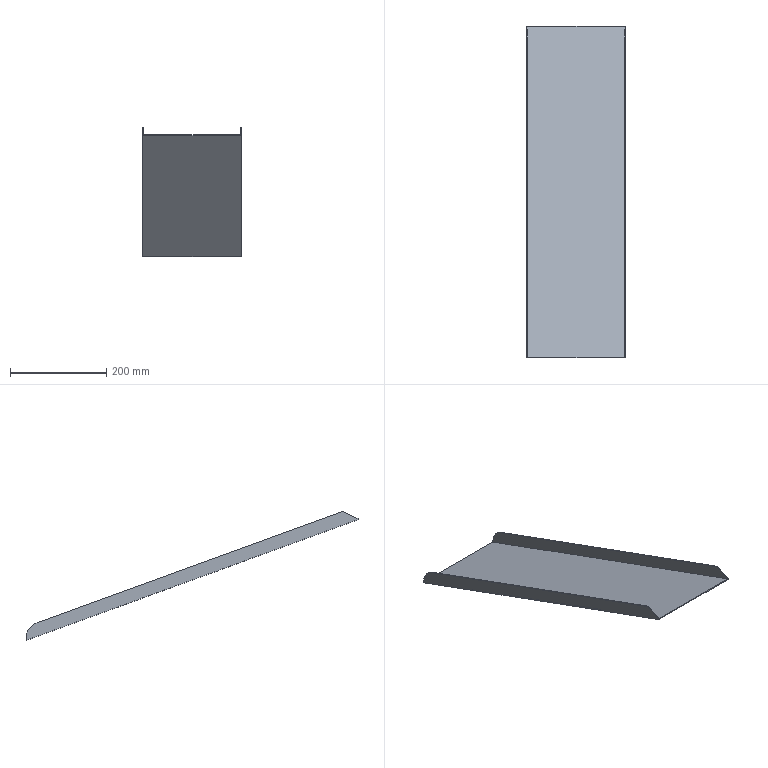Part | NX | features solid 2 | 1 solid | 14 faces | box 205 x 690 x 268.21 mm | volume 372341 mm3 | plane 12 | cylinder 2 | commonest cylinder face diameters 70 x2
STEP:
#1=CARTESIAN_POINT('',(-622.,620.,-449.011));
#2=VERTEX_POINT('',#1);
#3=CARTESIAN_POINT('',(-823.,620.,-449.011));
#4=VERTEX_POINT('',#3);
#5=CARTESIAN_POINT('',(-620.,620.,-449.011));
#6=DIRECTION('',(-1.,0.,0.));
#7=VECTOR('',#6,1000.);
#8=LINE('',#5,#7);
#9=EDGE_CURVE('',#2,#4,#8,.T.);
#10=ORIENTED_EDGE('',*,*,#9,.T.);
#11=CARTESIAN_POINT('',(-823.,-70.,-197.872));
#12=VERTEX_POINT('',#11);
#13=CARTESIAN_POINT('',(-823.,-70.,-197.872));
#14=DIRECTION('',(0.,0.9397,-0.342));
#15=VECTOR('',#14,1000.);
#16=LINE('',#13,#15);
#17=EDGE_CURVE('',#12,#4,#16,.T.);
#18=ORIENTED_EDGE('',*,*,#17,.F.);
#19=CARTESIAN_POINT('',(-622.,-70.,-197.872));
#20=VERTEX_POINT('',#19);
#21=CARTESIAN_POINT('',(-620.,-70.,-197.872));
#22=DIRECTION('',(1.,0.,0.));
#23=VECTOR('',#22,1000.);
#24=LINE('',#21,#23);
#25=EDGE_CURVE('',#20,#12,#24,.F.);
#26=ORIENTED_EDGE('',*,*,#25,.F.);
#27=CARTESIAN_POINT('',(-622.,-70.,-197.872));
#28=DIRECTION('',(0.,0.9397,-0.342));
#29=VECTOR('',#28,1000.);
#30=LINE('',#27,#29);
#31=EDGE_CURVE('',#20,#2,#30,.T.);
#32=ORIENTED_EDGE('',*,*,#31,.T.);
#33=EDGE_LOOP('',(#10,#18,#26,#32));
#34=FACE_BOUND('',#33,.T.);
#35=CARTESIAN_POINT('',(-620.,-69.316,-198.121));
#36=DIRECTION('',(0.,-0.342,-0.9397));
#37=DIRECTION('',(-1.,0.,0.));
#38=AXIS2_PLACEMENT_3D('',#35,#36,#37);
#39=PLANE('',#38);
#40=ADVANCED_FACE('',(#34),#39,.F.);
#41=CARTESIAN_POINT('',(-622.,620.,-446.914));
#42=VERTEX_POINT('',#41);
#43=CARTESIAN_POINT('',(-622.,620.,-570.));
#44=DIRECTION('',(0.,0.,1.));
#45=VECTOR('',#44,1000.);
#46=LINE('',#43,#45);
#47=EDGE_CURVE('',#2,#42,#46,.T.);
#48=ORIENTED_EDGE('',*,*,#47,.T.);
#49=CARTESIAN_POINT('',(-620.,620.,-446.914));
#50=VERTEX_POINT('',#49);
#51=CARTESIAN_POINT('',(285.,620.,-446.914));
#52=DIRECTION('',(-1.,0.,0.));
#53=VECTOR('',#52,1000.);
#54=LINE('',#51,#53);
#55=EDGE_CURVE('',#42,#50,#54,.F.);
#56=ORIENTED_EDGE('',*,*,#55,.T.);
#57=CARTESIAN_POINT('',(-620.,620.,-451.139));
#58=VERTEX_POINT('',#57);
#59=CARTESIAN_POINT('',(-620.,620.,-570.));
#60=DIRECTION('',(0.,0.,-1.));
#61=VECTOR('',#60,1000.);
#62=LINE('',#59,#61);
#63=EDGE_CURVE('',#50,#58,#62,.T.);
#64=ORIENTED_EDGE('',*,*,#63,.T.);
#65=CARTESIAN_POINT('',(-825.,620.,-451.139));
#66=VERTEX_POINT('',#65);
#67=CARTESIAN_POINT('',(-620.,620.,-451.139));
#68=DIRECTION('',(-1.,0.,0.));
#69=VECTOR('',#68,1000.);
#70=LINE('',#67,#69);
#71=EDGE_CURVE('',#58,#66,#70,.T.);
#72=ORIENTED_EDGE('',*,*,#71,.T.);
#73=CARTESIAN_POINT('',(-825.,620.,-446.914));
#74=VERTEX_POINT('',#73);
#75=CARTESIAN_POINT('',(-825.,620.,-570.));
#76=DIRECTION('',(0.,0.,-1.));
#77=VECTOR('',#76,1000.);
#78=LINE('',#75,#77);
#79=EDGE_CURVE('',#74,#66,#78,.T.);
#80=ORIENTED_EDGE('',*,*,#79,.F.);
#81=CARTESIAN_POINT('',(-823.,620.,-446.914));
#82=VERTEX_POINT('',#81);
#83=CARTESIAN_POINT('',(285.,620.,-446.914));
#84=DIRECTION('',(-1.,0.,0.));
#85=VECTOR('',#84,1000.);
#86=LINE('',#83,#85);
#87=EDGE_CURVE('',#74,#82,#86,.F.);
#88=ORIENTED_EDGE('',*,*,#87,.T.);
#89=CARTESIAN_POINT('',(-823.,620.,-570.));
#90=DIRECTION('',(0.,0.,1.));
#91=VECTOR('',#90,1000.);
#92=LINE('',#89,#91);
#93=EDGE_CURVE('',#4,#82,#92,.T.);
#94=ORIENTED_EDGE('',*,*,#93,.F.);
#95=ORIENTED_EDGE('',*,*,#9,.F.);
#96=EDGE_LOOP('',(#48,#56,#64,#72,#80,#88,#94,#95));
#97=FACE_BOUND('',#96,.T.);
#98=CARTESIAN_POINT('',(285.,620.,-570.));
#99=DIRECTION('',(0.,-1.,0.));
#100=DIRECTION('',(-1.,0.,0.));
#101=AXIS2_PLACEMENT_3D('',#98,#99,#100);
#102=PLANE('',#101);
#103=ADVANCED_FACE('',(#97),#102,.F.);
#104=CARTESIAN_POINT('',(-620.,-37.957,-182.93));
#105=VERTEX_POINT('',#104);
#106=CARTESIAN_POINT('',(-620.,596.971,-414.025));
#107=VERTEX_POINT('',#106);
#108=CARTESIAN_POINT('',(-620.,-61.449,-174.379));
#109=DIRECTION('',(0.,0.9397,-0.342));
#110=VECTOR('',#109,1000.);
#111=LINE('',#108,#110);
#112=EDGE_CURVE('',#105,#107,#111,.T.);
#113=ORIENTED_EDGE('',*,*,#112,.F.);
#114=CARTESIAN_POINT('',(-620.,-70.,-197.872));
#115=VERTEX_POINT('',#114);
#116=CARTESIAN_POINT('',(-620.,-70.,-197.872));
#117=DIRECTION('',(0.,0.9063,0.4226));
#118=VECTOR('',#117,1000.);
#119=LINE('',#116,#118);
#120=EDGE_CURVE('',#105,#115,#119,.F.);
#121=ORIENTED_EDGE('',*,*,#120,.T.);
#122=CARTESIAN_POINT('',(-620.,-70.,-200.));
#123=VERTEX_POINT('',#122);
#124=CARTESIAN_POINT('',(-620.,-70.,0.000000753));
#125=DIRECTION('',(0.,0.,1.));
#126=VECTOR('',#125,1000.);
#127=LINE('',#124,#126);
#128=EDGE_CURVE('',#115,#123,#127,.F.);
#129=ORIENTED_EDGE('',*,*,#128,.T.);
#130=CARTESIAN_POINT('',(-620.,-70.,-200.));
#131=DIRECTION('',(0.,0.9397,-0.342));
#132=VECTOR('',#131,1000.);
#133=LINE('',#130,#132);
#134=EDGE_CURVE('',#123,#58,#133,.T.);
#135=ORIENTED_EDGE('',*,*,#134,.T.);
#136=ORIENTED_EDGE('',*,*,#63,.F.);
#137=CARTESIAN_POINT('',(-620.,585.,-446.914));
#138=DIRECTION('',(-1.,0.,0.));
#139=DIRECTION('',(0.,0.,1.));
#140=AXIS2_PLACEMENT_3D('',#137,#138,#139);
#141=CIRCLE('',#140,35.);
#142=EDGE_CURVE('',#50,#107,#141,.F.);
#143=ORIENTED_EDGE('',*,*,#142,.T.);
#144=EDGE_LOOP('',(#113,#121,#129,#135,#136,#143));
#145=FACE_BOUND('',#144,.T.);
#146=CARTESIAN_POINT('',(-620.,-69.316,-198.121));
#147=DIRECTION('',(-1.,0.,0.));
#148=DIRECTION('',(0.,0.,1.));
#149=AXIS2_PLACEMENT_3D('',#146,#147,#148);
#150=PLANE('',#149);
#151=ADVANCED_FACE('',(#145),#150,.F.);
#152=CARTESIAN_POINT('',(-825.,-70.,-200.));
#153=VERTEX_POINT('',#152);
#154=CARTESIAN_POINT('',(-620.,-70.,-200.));
#155=DIRECTION('',(1.,0.,0.));
#156=VECTOR('',#155,1000.);
#157=LINE('',#154,#156);
#158=EDGE_CURVE('',#123,#153,#157,.F.);
#159=ORIENTED_EDGE('',*,*,#158,.F.);
#160=ORIENTED_EDGE('',*,*,#128,.F.);
#161=CARTESIAN_POINT('',(-620.,-70.,-197.872));
#162=DIRECTION('',(1.,0.,0.));
#163=VECTOR('',#162,1000.);
#164=LINE('',#161,#163);
#165=EDGE_CURVE('',#115,#20,#164,.F.);
#166=ORIENTED_EDGE('',*,*,#165,.T.);
#167=ORIENTED_EDGE('',*,*,#25,.T.);
#168=CARTESIAN_POINT('',(-825.,-70.,-197.872));
#169=VERTEX_POINT('',#168);
#170=CARTESIAN_POINT('',(-873.,-70.,-197.872));
#171=DIRECTION('',(1.,0.,0.));
#172=VECTOR('',#171,1000.);
#173=LINE('',#170,#172);
#174=EDGE_CURVE('',#12,#169,#173,.F.);
#175=ORIENTED_EDGE('',*,*,#174,.T.);
#176=CARTESIAN_POINT('',(-825.,-70.,0.000000798));
#177=DIRECTION('',(0.,0.,1.));
#178=VECTOR('',#177,1000.);
#179=LINE('',#176,#178);
#180=EDGE_CURVE('',#169,#153,#179,.F.);
#181=ORIENTED_EDGE('',*,*,#180,.T.);
#182=EDGE_LOOP('',(#159,#160,#166,#167,#175,#181));
#183=FACE_BOUND('',#182,.T.);
#184=CARTESIAN_POINT('',(2775.,-70.,0.000000013));
#185=DIRECTION('',(0.,1.,0.));
#186=DIRECTION('',(0.,0.,1.));
#187=AXIS2_PLACEMENT_3D('',#184,#185,#186);
#188=PLANE('',#187);
#189=ADVANCED_FACE('',(#183),#188,.F.);
#190=ORIENTED_EDGE('',*,*,#180,.F.);
#191=CARTESIAN_POINT('',(-825.,-37.957,-182.93));
#192=VERTEX_POINT('',#191);
#193=CARTESIAN_POINT('',(-825.,-69.533,-197.654));
#194=DIRECTION('',(0.,-0.9063,-0.4226));
#195=VECTOR('',#194,1000.);
#196=LINE('',#193,#195);
#197=EDGE_CURVE('',#169,#192,#196,.F.);
#198=ORIENTED_EDGE('',*,*,#197,.T.);
#199=CARTESIAN_POINT('',(-825.,596.971,-414.025));
#200=VERTEX_POINT('',#199);
#201=CARTESIAN_POINT('',(-825.,-61.449,-174.379));
#202=DIRECTION('',(0.,0.9397,-0.342));
#203=VECTOR('',#202,1000.);
#204=LINE('',#201,#203);
#205=EDGE_CURVE('',#192,#200,#204,.T.);
#206=ORIENTED_EDGE('',*,*,#205,.T.);
#207=CARTESIAN_POINT('',(-825.,585.,-446.914));
#208=DIRECTION('',(-1.,0.,0.));
#209=DIRECTION('',(0.,0.,1.));
#210=AXIS2_PLACEMENT_3D('',#207,#208,#209);
#211=CIRCLE('',#210,35.);
#212=EDGE_CURVE('',#200,#74,#211,.T.);
#213=ORIENTED_EDGE('',*,*,#212,.T.);
#214=ORIENTED_EDGE('',*,*,#79,.T.);
#215=CARTESIAN_POINT('',(-825.,-70.,-200.));
#216=DIRECTION('',(0.,0.9397,-0.342));
#217=VECTOR('',#216,1000.);
#218=LINE('',#215,#217);
#219=EDGE_CURVE('',#153,#66,#218,.T.);
#220=ORIENTED_EDGE('',*,*,#219,.F.);
#221=EDGE_LOOP('',(#190,#198,#206,#213,#214,#220));
#222=FACE_BOUND('',#221,.T.);
#223=CARTESIAN_POINT('',(-825.,-69.316,-198.121));
#224=DIRECTION('',(-1.,0.,0.));
#225=DIRECTION('',(0.,0.,1.));
#226=AXIS2_PLACEMENT_3D('',#223,#224,#225);
#227=PLANE('',#226);
#228=ADVANCED_FACE('',(#222),#227,.T.);
#229=ORIENTED_EDGE('',*,*,#71,.F.);
#230=ORIENTED_EDGE('',*,*,#134,.F.);
#231=ORIENTED_EDGE('',*,*,#158,.T.);
#232=ORIENTED_EDGE('',*,*,#219,.T.);
#233=EDGE_LOOP('',(#229,#230,#231,#232));
#234=FACE_BOUND('',#233,.T.);
#235=CARTESIAN_POINT('',(-620.,-70.,-200.));
#236=DIRECTION('',(0.,-0.342,-0.9397));
#237=DIRECTION('',(-1.,0.,0.));
#238=AXIS2_PLACEMENT_3D('',#235,#236,#237);
#239=PLANE('',#238);
#240=ADVANCED_FACE('',(#234),#239,.T.);
#241=CARTESIAN_POINT('',(-622.,-37.957,-182.93));
#242=VERTEX_POINT('',#241);
#243=CARTESIAN_POINT('',(-622.,596.971,-414.025));
#244=VERTEX_POINT('',#243);
#245=CARTESIAN_POINT('',(-622.,-61.449,-174.379));
#246=DIRECTION('',(0.,0.9397,-0.342));
#247=VECTOR('',#246,1000.);
#248=LINE('',#245,#247);
#249=EDGE_CURVE('',#242,#244,#248,.T.);
#250=ORIENTED_EDGE('',*,*,#249,.F.);
#251=CARTESIAN_POINT('',(-620.,-37.957,-182.93));
#252=DIRECTION('',(1.,0.,0.));
#253=VECTOR('',#252,1000.);
#254=LINE('',#251,#253);
#255=EDGE_CURVE('',#242,#105,#254,.T.);
#256=ORIENTED_EDGE('',*,*,#255,.T.);
#257=ORIENTED_EDGE('',*,*,#112,.T.);
#258=CARTESIAN_POINT('',(-620.,596.971,-414.025));
#259=DIRECTION('',(-1.,0.,0.));
#260=VECTOR('',#259,1000.);
#261=LINE('',#258,#260);
#262=EDGE_CURVE('',#107,#244,#261,.T.);
#263=ORIENTED_EDGE('',*,*,#262,.T.);
#264=EDGE_LOOP('',(#250,#256,#257,#263));
#265=FACE_BOUND('',#264,.T.);
#266=CARTESIAN_POINT('',(-620.,-61.449,-174.379));
#267=DIRECTION('',(0.,-0.342,-0.9397));
#268=DIRECTION('',(0.,0.9397,-0.342));
#269=AXIS2_PLACEMENT_3D('',#266,#267,#268);
#270=PLANE('',#269);
#271=ADVANCED_FACE('',(#265),#270,.F.);
#272=ORIENTED_EDGE('',*,*,#31,.F.);
#273=CARTESIAN_POINT('',(-622.,-70.,-197.872));
#274=DIRECTION('',(0.,-0.9063,-0.4226));
#275=VECTOR('',#274,1000.);
#276=LINE('',#273,#275);
#277=EDGE_CURVE('',#20,#242,#276,.F.);
#278=ORIENTED_EDGE('',*,*,#277,.T.);
#279=ORIENTED_EDGE('',*,*,#249,.T.);
#280=CARTESIAN_POINT('',(-622.,585.,-446.914));
#281=DIRECTION('',(1.,0.,0.));
#282=DIRECTION('',(0.,0.,-1.));
#283=AXIS2_PLACEMENT_3D('',#280,#281,#282);
#284=CIRCLE('',#283,35.);
#285=EDGE_CURVE('',#244,#42,#284,.F.);
#286=ORIENTED_EDGE('',*,*,#285,.T.);
#287=ORIENTED_EDGE('',*,*,#47,.F.);
#288=EDGE_LOOP('',(#272,#278,#279,#286,#287));
#289=FACE_BOUND('',#288,.T.);
#290=CARTESIAN_POINT('',(-622.,-70.,-197.872));
#291=DIRECTION('',(1.,0.,0.));
#292=DIRECTION('',(0.,0.,-1.));
#293=AXIS2_PLACEMENT_3D('',#290,#291,#292);
#294=PLANE('',#293);
#295=ADVANCED_FACE('',(#289),#294,.F.);
#296=ORIENTED_EDGE('',*,*,#205,.F.);
#297=CARTESIAN_POINT('',(-823.,-37.957,-182.93));
#298=VERTEX_POINT('',#297);
#299=CARTESIAN_POINT('',(-873.,-37.957,-182.93));
#300=DIRECTION('',(1.,0.,0.));
#301=VECTOR('',#300,1000.);
#302=LINE('',#299,#301);
#303=EDGE_CURVE('',#192,#298,#302,.T.);
#304=ORIENTED_EDGE('',*,*,#303,.T.);
#305=CARTESIAN_POINT('',(-823.,596.971,-414.025));
#306=VERTEX_POINT('',#305);
#307=CARTESIAN_POINT('',(-823.,-61.449,-174.379));
#308=DIRECTION('',(0.,0.9397,-0.342));
#309=VECTOR('',#308,1000.);
#310=LINE('',#307,#309);
#311=EDGE_CURVE('',#298,#306,#310,.T.);
#312=ORIENTED_EDGE('',*,*,#311,.T.);
#313=CARTESIAN_POINT('',(-873.,596.971,-414.025));
#314=DIRECTION('',(-1.,0.,0.));
#315=VECTOR('',#314,1000.);
#316=LINE('',#313,#315);
#317=EDGE_CURVE('',#306,#200,#316,.T.);
#318=ORIENTED_EDGE('',*,*,#317,.T.);
#319=EDGE_LOOP('',(#296,#304,#312,#318));
#320=FACE_BOUND('',#319,.T.);
#321=CARTESIAN_POINT('',(-873.,-61.449,-174.379));
#322=DIRECTION('',(0.,-0.342,-0.9397));
#323=DIRECTION('',(0.,0.9397,-0.342));
#324=AXIS2_PLACEMENT_3D('',#321,#322,#323);
#325=PLANE('',#324);
#326=ADVANCED_FACE('',(#320),#325,.F.);
#327=ORIENTED_EDGE('',*,*,#311,.F.);
#328=CARTESIAN_POINT('',(-823.,-70.,-197.872));
#329=DIRECTION('',(0.,0.9063,0.4226));
#330=VECTOR('',#329,1000.);
#331=LINE('',#328,#330);
#332=EDGE_CURVE('',#298,#12,#331,.F.);
#333=ORIENTED_EDGE('',*,*,#332,.T.);
#334=ORIENTED_EDGE('',*,*,#17,.T.);
#335=ORIENTED_EDGE('',*,*,#93,.T.);
#336=CARTESIAN_POINT('',(-823.,585.,-446.914));
#337=DIRECTION('',(1.,0.,0.));
#338=DIRECTION('',(0.,0.,-1.));
#339=AXIS2_PLACEMENT_3D('',#336,#337,#338);
#340=CIRCLE('',#339,35.);
#341=EDGE_CURVE('',#82,#306,#340,.T.);
#342=ORIENTED_EDGE('',*,*,#341,.T.);
#343=EDGE_LOOP('',(#327,#333,#334,#335,#342));
#344=FACE_BOUND('',#343,.T.);
#345=CARTESIAN_POINT('',(-823.,-70.,-197.872));
#346=DIRECTION('',(1.,0.,0.));
#347=DIRECTION('',(0.,0.,-1.));
#348=AXIS2_PLACEMENT_3D('',#345,#346,#347);
#349=PLANE('',#348);
#350=ADVANCED_FACE('',(#344),#349,.T.);
#351=ORIENTED_EDGE('',*,*,#341,.F.);
#352=ORIENTED_EDGE('',*,*,#87,.F.);
#353=ORIENTED_EDGE('',*,*,#212,.F.);
#354=ORIENTED_EDGE('',*,*,#317,.F.);
#355=EDGE_LOOP('',(#351,#352,#353,#354));
#356=FACE_BOUND('',#355,.T.);
#357=CARTESIAN_POINT('',(-873.,585.,-446.914));
#358=DIRECTION('',(-1.,0.,0.));
#359=DIRECTION('',(0.,0.,1.));
#360=AXIS2_PLACEMENT_3D('',#357,#358,#359);
#361=CYLINDRICAL_SURFACE('',#360,35.);
#362=ADVANCED_FACE('',(#356),#361,.T.);
#363=ORIENTED_EDGE('',*,*,#142,.F.);
#364=ORIENTED_EDGE('',*,*,#55,.F.);
#365=ORIENTED_EDGE('',*,*,#285,.F.);
#366=ORIENTED_EDGE('',*,*,#262,.F.);
#367=EDGE_LOOP('',(#363,#364,#365,#366));
#368=FACE_BOUND('',#367,.T.);
#369=CARTESIAN_POINT('',(-620.,585.,-446.914));
#370=DIRECTION('',(-1.,0.,0.));
#371=DIRECTION('',(0.,0.,1.));
#372=AXIS2_PLACEMENT_3D('',#369,#370,#371);
#373=CYLINDRICAL_SURFACE('',#372,35.);
#374=ADVANCED_FACE('',(#368),#373,.T.);
#375=ORIENTED_EDGE('',*,*,#332,.F.);
#376=ORIENTED_EDGE('',*,*,#303,.F.);
#377=ORIENTED_EDGE('',*,*,#197,.F.);
#378=ORIENTED_EDGE('',*,*,#174,.F.);
#379=EDGE_LOOP('',(#375,#376,#377,#378));
#380=FACE_BOUND('',#379,.T.);
#381=CARTESIAN_POINT('',(-873.,-70.,-197.872));
#382=DIRECTION('',(0.,0.4226,-0.9063));
#383=DIRECTION('',(0.,0.9063,0.4226));
#384=AXIS2_PLACEMENT_3D('',#381,#382,#383);
#385=PLANE('',#384);
#386=ADVANCED_FACE('',(#380),#385,.F.);
#387=ORIENTED_EDGE('',*,*,#120,.F.);
#388=ORIENTED_EDGE('',*,*,#255,.F.);
#389=ORIENTED_EDGE('',*,*,#277,.F.);
#390=ORIENTED_EDGE('',*,*,#165,.F.);
#391=EDGE_LOOP('',(#387,#388,#389,#390));
#392=FACE_BOUND('',#391,.T.);
#393=CARTESIAN_POINT('',(-620.,-70.,-197.872));
#394=DIRECTION('',(0.,0.4226,-0.9063));
#395=DIRECTION('',(0.,0.9063,0.4226));
#396=AXIS2_PLACEMENT_3D('',#393,#394,#395);
#397=PLANE('',#396);
#398=ADVANCED_FACE('',(#392),#397,.F.);
#399=CLOSED_SHELL('',(#40,#103,#151,#189,#228,#240,#271,#295,#326,#350,#362,#374,#386,#398));
#400=MANIFOLD_SOLID_BREP('',#399);
#401=(LENGTH_UNIT()NAMED_UNIT(*)SI_UNIT(.MILLI.,.METRE.));
#402=UNCERTAINTY_MEASURE_WITH_UNIT(LENGTH_MEASURE(0.00001),#401,'','');
#403=(NAMED_UNIT(*)PLANE_ANGLE_UNIT()SI_UNIT($,.RADIAN.));
#404=(NAMED_UNIT(*)SI_UNIT($,.STERADIAN.)SOLID_ANGLE_UNIT());
#405=(GEOMETRIC_REPRESENTATION_CONTEXT(3)GLOBAL_UNCERTAINTY_ASSIGNED_CONTEXT((#402))GLOBAL_UNIT_ASSIGNED_CONTEXT((#401,#403,#404))REPRESENTATION_CONTEXT('',''));
#406=ADVANCED_BREP_SHAPE_REPRESENTATION('',(#400),#405);